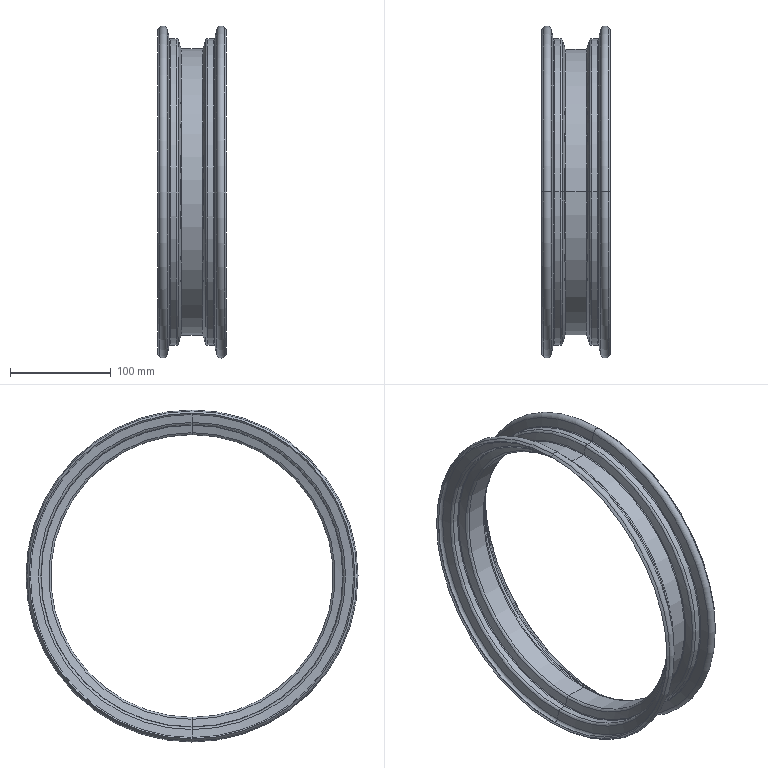Part | SolidWorks | features BaseBody 1 | 1 solid | 72 faces | box 67.896 x 329.277 x 329.277 mm | volume 165413 mm3 | torus 32 | cone 28 | cylinder 12 | commonest cylinder face diameters 300.503 x4 304 x4 280.5 x2 283.997 x2